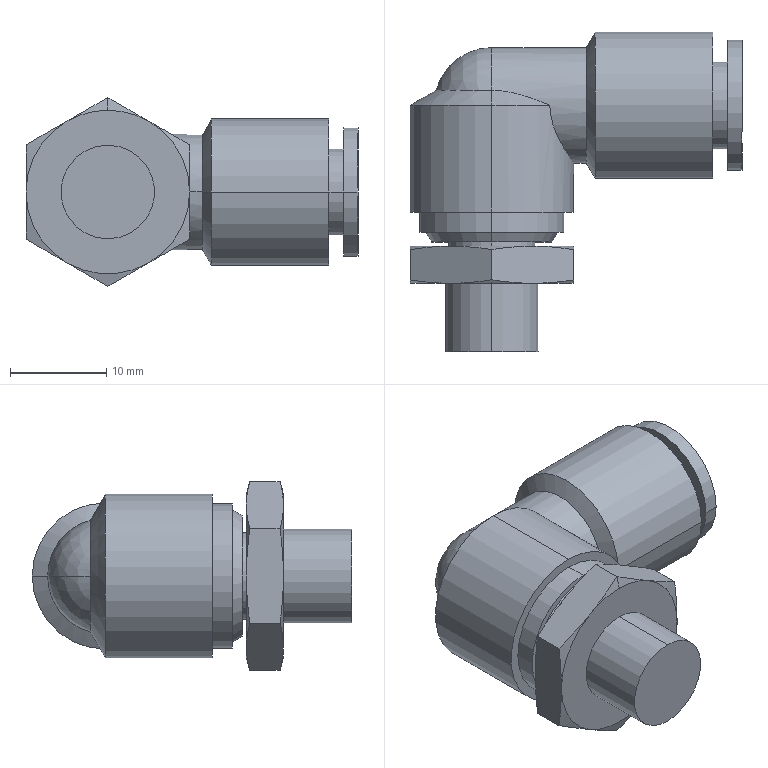Part | SolidWorks | features BaseBody 1 | 1 solid | 57 faces | box 34.5 x 33.2 x 19.63 mm | volume 7219 mm3 | cone 21 | cylinder 18 | plane 16 | sphere 2 | commonest cylinder face diameters 9 x4 8 x2 9.728 x2 12 x2 13.5 x2 15 x2